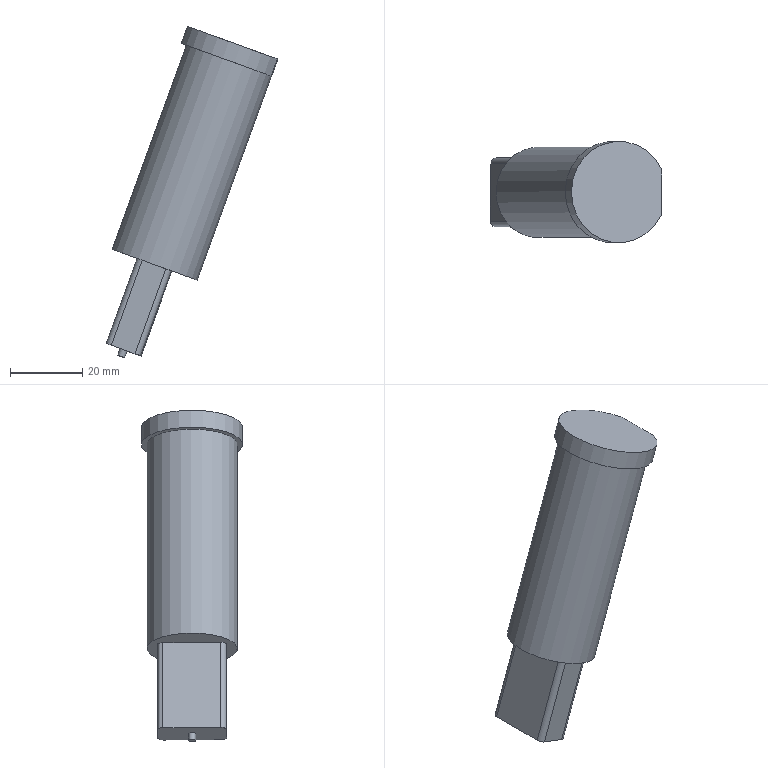Part | NX | features solid 2 | 1 solid | 17 faces | box 47.429 x 28 x 91.582 mm | volume 37175 mm3 | plane 10 | cylinder 7 | commonest cylinder face diameters 3 x4 2 x1 25 x1 28 x1